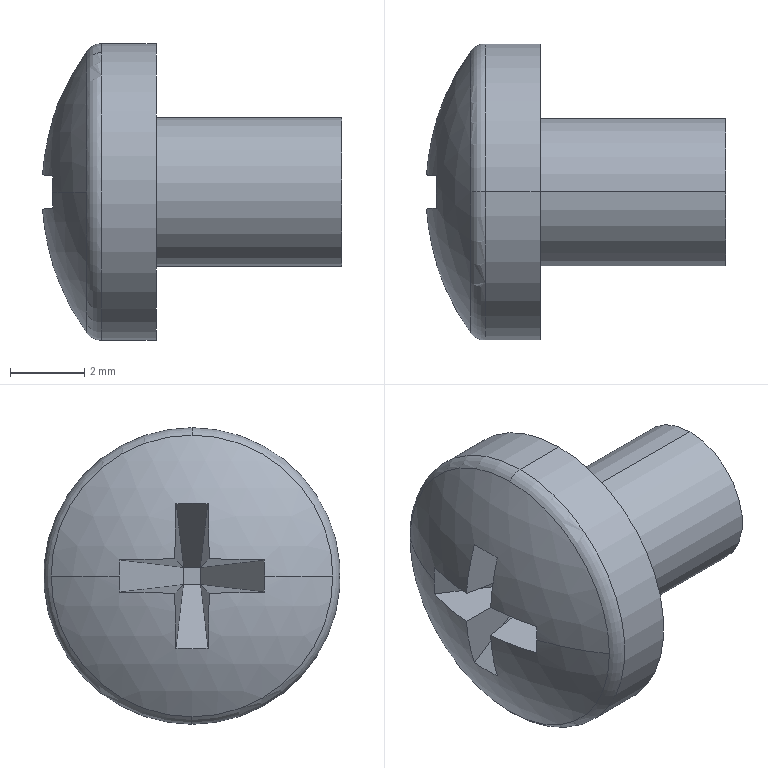Part | STEP file | B18.6.7M - M4 x 0.7 x 5 Type I Cross Recessed PHMS --5N | 1 solid | 23 faces | box 8.067 x 8 x 8 mm | volume 178.262 mm3 | plane 15 | cylinder 4 | torus 2 | sphere 2 | commonest cylinder face diameters 4 x2 8 x2